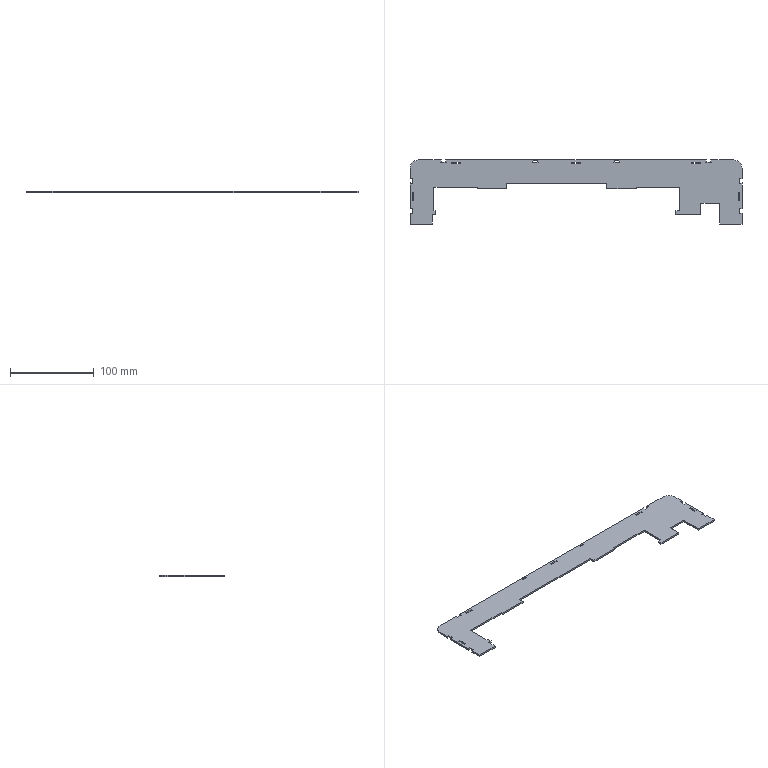Part | STEP file | xzz-002-1 | 1 solid | 82 faces | box 397.4 x 76.7 x 2 mm | volume 32215 mm3 | plane 80 | cylinder 2 | commonest cylinder face diameters 20 x2